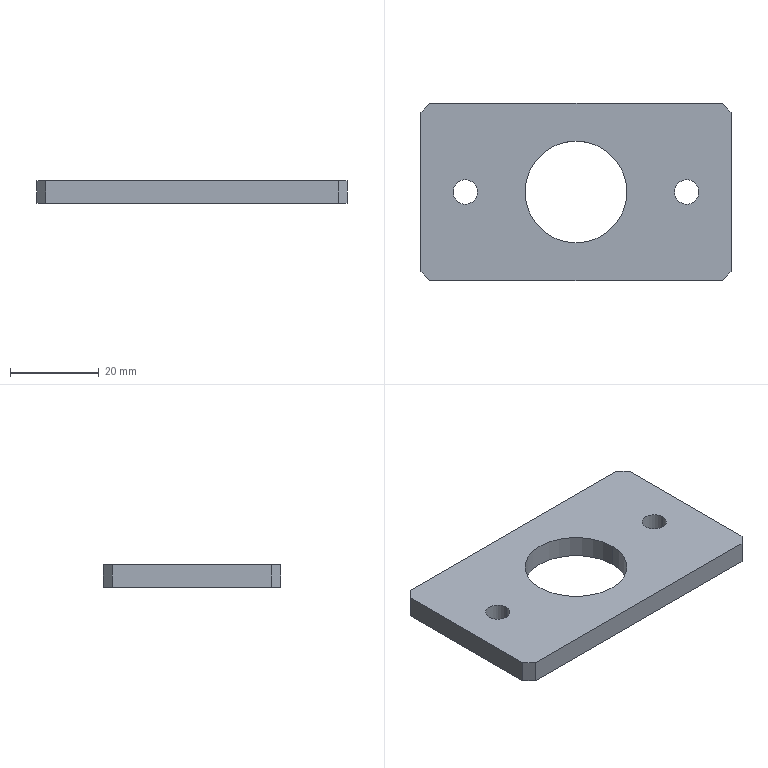Part | SolidWorks | features Chamfer 1, FlatPattern 1, HoleWzd 1, ICE 1, SMBaseFlange 1, SheetMetal 1 | 1 solid | 16 faces | box 70 x 40 x 5 mm | volume 11645 mm3 | plane 10 | cylinder 6 | commonest cylinder face diameters 5.5 x4 23 x2
STEP:
#1=CARTESIAN_POINT('',(22.25,0.,-5.));
#2=VERTEX_POINT('',#1);
#3=CARTESIAN_POINT('',(27.75,0.,-5.));
#4=VERTEX_POINT('',#3);
#5=CARTESIAN_POINT('',(25.,0.,-5.));
#6=DIRECTION('',(0.,0.,1.));
#7=DIRECTION('',(1.,0.,0.));
#8=AXIS2_PLACEMENT_3D('',#5,#6,#7);
#9=CIRCLE('',#8,2.75);
#10=EDGE_CURVE('',#2,#4,#9,.T.);
#11=ORIENTED_EDGE('',*,*,#10,.F.);
#12=CARTESIAN_POINT('',(22.25,0.,0.));
#13=VERTEX_POINT('',#12);
#14=CARTESIAN_POINT('',(22.25,0.,0.));
#15=DIRECTION('',(0.,0.,1.));
#16=VECTOR('',#15,1000.);
#17=LINE('',#14,#16);
#18=EDGE_CURVE('',#2,#13,#17,.T.);
#19=ORIENTED_EDGE('',*,*,#18,.T.);
#20=CARTESIAN_POINT('',(27.75,0.,0.));
#21=VERTEX_POINT('',#20);
#22=CARTESIAN_POINT('',(25.,0.,0.));
#23=DIRECTION('',(0.,0.,1.));
#24=DIRECTION('',(1.,0.,0.));
#25=AXIS2_PLACEMENT_3D('',#22,#23,#24);
#26=CIRCLE('',#25,2.75);
#27=EDGE_CURVE('',#13,#21,#26,.T.);
#28=ORIENTED_EDGE('',*,*,#27,.T.);
#29=CARTESIAN_POINT('',(27.75,0.,0.));
#30=DIRECTION('',(0.,0.,1.));
#31=VECTOR('',#30,1000.);
#32=LINE('',#29,#31);
#33=EDGE_CURVE('',#4,#21,#32,.T.);
#34=ORIENTED_EDGE('',*,*,#33,.F.);
#35=EDGE_LOOP('',(#11,#19,#28,#34));
#36=FACE_OUTER_BOUND('',#35,.T.);
#37=CARTESIAN_POINT('',(25.,0.,0.));
#38=DIRECTION('',(0.,0.,1.));
#39=DIRECTION('',(1.,0.,0.));
#40=AXIS2_PLACEMENT_3D('',#37,#38,#39);
#41=CYLINDRICAL_SURFACE('',#40,2.75);
#42=ADVANCED_FACE('',(#36),#41,.F.);
#43=CARTESIAN_POINT('',(-27.75,0.,-5.));
#44=VERTEX_POINT('',#43);
#45=CARTESIAN_POINT('',(-22.25,0.,-5.));
#46=VERTEX_POINT('',#45);
#47=CARTESIAN_POINT('',(-25.,0.,-5.));
#48=DIRECTION('',(0.,0.,1.));
#49=DIRECTION('',(1.,0.,0.));
#50=AXIS2_PLACEMENT_3D('',#47,#48,#49);
#51=CIRCLE('',#50,2.75);
#52=EDGE_CURVE('',#44,#46,#51,.T.);
#53=ORIENTED_EDGE('',*,*,#52,.F.);
#54=CARTESIAN_POINT('',(-27.75,0.,0.));
#55=VERTEX_POINT('',#54);
#56=CARTESIAN_POINT('',(-27.75,0.,0.));
#57=DIRECTION('',(0.,0.,1.));
#58=VECTOR('',#57,1000.);
#59=LINE('',#56,#58);
#60=EDGE_CURVE('',#44,#55,#59,.T.);
#61=ORIENTED_EDGE('',*,*,#60,.T.);
#62=CARTESIAN_POINT('',(-22.25,0.,0.));
#63=VERTEX_POINT('',#62);
#64=CARTESIAN_POINT('',(-25.,0.,0.));
#65=DIRECTION('',(0.,0.,1.));
#66=DIRECTION('',(1.,0.,0.));
#67=AXIS2_PLACEMENT_3D('',#64,#65,#66);
#68=CIRCLE('',#67,2.75);
#69=EDGE_CURVE('',#55,#63,#68,.T.);
#70=ORIENTED_EDGE('',*,*,#69,.T.);
#71=CARTESIAN_POINT('',(-22.25,0.,0.));
#72=DIRECTION('',(0.,0.,1.));
#73=VECTOR('',#72,1000.);
#74=LINE('',#71,#73);
#75=EDGE_CURVE('',#46,#63,#74,.T.);
#76=ORIENTED_EDGE('',*,*,#75,.F.);
#77=EDGE_LOOP('',(#53,#61,#70,#76));
#78=FACE_OUTER_BOUND('',#77,.T.);
#79=CARTESIAN_POINT('',(-25.,0.,0.));
#80=DIRECTION('',(0.,0.,1.));
#81=DIRECTION('',(1.,0.,0.));
#82=AXIS2_PLACEMENT_3D('',#79,#80,#81);
#83=CYLINDRICAL_SURFACE('',#82,2.75);
#84=ADVANCED_FACE('',(#78),#83,.F.);
#85=CARTESIAN_POINT('',(-11.5,0.,-5.));
#86=VERTEX_POINT('',#85);
#87=CARTESIAN_POINT('',(11.5,0.,-5.));
#88=VERTEX_POINT('',#87);
#89=CARTESIAN_POINT('',(0.,0.,-5.));
#90=DIRECTION('',(0.,0.,1.));
#91=DIRECTION('',(1.,0.,0.));
#92=AXIS2_PLACEMENT_3D('',#89,#90,#91);
#93=CIRCLE('',#92,11.5);
#94=EDGE_CURVE('',#86,#88,#93,.T.);
#95=ORIENTED_EDGE('',*,*,#94,.F.);
#96=CARTESIAN_POINT('',(-11.5,0.,0.));
#97=VERTEX_POINT('',#96);
#98=CARTESIAN_POINT('',(-11.5,0.,-10.));
#99=DIRECTION('',(0.,0.,1.));
#100=VECTOR('',#99,1000.);
#101=LINE('',#98,#100);
#102=EDGE_CURVE('',#86,#97,#101,.T.);
#103=ORIENTED_EDGE('',*,*,#102,.T.);
#104=CARTESIAN_POINT('',(11.5,0.,0.));
#105=VERTEX_POINT('',#104);
#106=CARTESIAN_POINT('',(0.,0.,0.));
#107=DIRECTION('',(0.,0.,1.));
#108=DIRECTION('',(1.,0.,0.));
#109=AXIS2_PLACEMENT_3D('',#106,#107,#108);
#110=CIRCLE('',#109,11.5);
#111=EDGE_CURVE('',#97,#105,#110,.T.);
#112=ORIENTED_EDGE('',*,*,#111,.T.);
#113=CARTESIAN_POINT('',(11.5,0.,-10.));
#114=DIRECTION('',(0.,0.,1.));
#115=VECTOR('',#114,1000.);
#116=LINE('',#113,#115);
#117=EDGE_CURVE('',#88,#105,#116,.T.);
#118=ORIENTED_EDGE('',*,*,#117,.F.);
#119=EDGE_LOOP('',(#95,#103,#112,#118));
#120=FACE_OUTER_BOUND('',#119,.T.);
#121=CARTESIAN_POINT('',(0.,0.,-10.));
#122=DIRECTION('',(0.,0.,1.));
#123=DIRECTION('',(1.,0.,0.));
#124=AXIS2_PLACEMENT_3D('',#121,#122,#123);
#125=CYLINDRICAL_SURFACE('',#124,11.5);
#126=ADVANCED_FACE('',(#120),#125,.F.);
#127=CARTESIAN_POINT('',(35.,-18.,-5.));
#128=VERTEX_POINT('',#127);
#129=CARTESIAN_POINT('',(35.,18.,-5.));
#130=VERTEX_POINT('',#129);
#131=CARTESIAN_POINT('',(35.,20.,-5.));
#132=DIRECTION('',(0.,1.,0.));
#133=VECTOR('',#132,1000.);
#134=LINE('',#131,#133);
#135=EDGE_CURVE('',#128,#130,#134,.T.);
#136=ORIENTED_EDGE('',*,*,#135,.T.);
#137=CARTESIAN_POINT('',(35.,18.,0.));
#138=VERTEX_POINT('',#137);
#139=CARTESIAN_POINT('',(35.,18.,-5.));
#140=DIRECTION('',(0.,0.,1.));
#141=VECTOR('',#140,1000.);
#142=LINE('',#139,#141);
#143=EDGE_CURVE('',#130,#138,#142,.T.);
#144=ORIENTED_EDGE('',*,*,#143,.T.);
#145=CARTESIAN_POINT('',(35.,-18.,0.));
#146=VERTEX_POINT('',#145);
#147=CARTESIAN_POINT('',(35.,20.,0.));
#148=DIRECTION('',(0.,1.,0.));
#149=VECTOR('',#148,1000.);
#150=LINE('',#147,#149);
#151=EDGE_CURVE('',#146,#138,#150,.T.);
#152=ORIENTED_EDGE('',*,*,#151,.F.);
#153=CARTESIAN_POINT('',(35.,-18.,-5.));
#154=DIRECTION('',(0.,0.,-1.));
#155=VECTOR('',#154,1000.);
#156=LINE('',#153,#155);
#157=EDGE_CURVE('',#146,#128,#156,.T.);
#158=ORIENTED_EDGE('',*,*,#157,.T.);
#159=EDGE_LOOP('',(#136,#144,#152,#158));
#160=FACE_OUTER_BOUND('',#159,.T.);
#161=CARTESIAN_POINT('',(35.,20.,-5.));
#162=DIRECTION('',(1.,0.,0.));
#163=DIRECTION('',(0.,1.,0.));
#164=AXIS2_PLACEMENT_3D('',#161,#162,#163);
#165=PLANE('',#164);
#166=ADVANCED_FACE('',(#160),#165,.T.);
#167=CARTESIAN_POINT('',(-33.,-20.,0.));
#168=VERTEX_POINT('',#167);
#169=CARTESIAN_POINT('',(33.,-20.,0.));
#170=VERTEX_POINT('',#169);
#171=CARTESIAN_POINT('',(-35.,-20.,0.));
#172=DIRECTION('',(1.,0.,0.));
#173=VECTOR('',#172,1000.);
#174=LINE('',#171,#173);
#175=EDGE_CURVE('',#168,#170,#174,.T.);
#176=ORIENTED_EDGE('',*,*,#175,.F.);
#177=CARTESIAN_POINT('',(-33.,-20.,-5.));
#178=VERTEX_POINT('',#177);
#179=CARTESIAN_POINT('',(-33.,-20.,-5.));
#180=DIRECTION('',(0.,0.,-1.));
#181=VECTOR('',#180,1000.);
#182=LINE('',#179,#181);
#183=EDGE_CURVE('',#168,#178,#182,.T.);
#184=ORIENTED_EDGE('',*,*,#183,.T.);
#185=CARTESIAN_POINT('',(33.,-20.,-5.));
#186=VERTEX_POINT('',#185);
#187=CARTESIAN_POINT('',(-35.,-20.,-5.));
#188=DIRECTION('',(1.,0.,0.));
#189=VECTOR('',#188,1000.);
#190=LINE('',#187,#189);
#191=EDGE_CURVE('',#178,#186,#190,.T.);
#192=ORIENTED_EDGE('',*,*,#191,.T.);
#193=CARTESIAN_POINT('',(33.,-20.,-5.));
#194=DIRECTION('',(0.,0.,1.));
#195=VECTOR('',#194,1000.);
#196=LINE('',#193,#195);
#197=EDGE_CURVE('',#186,#170,#196,.T.);
#198=ORIENTED_EDGE('',*,*,#197,.T.);
#199=EDGE_LOOP('',(#176,#184,#192,#198));
#200=FACE_OUTER_BOUND('',#199,.T.);
#201=CARTESIAN_POINT('',(-35.,-20.,-5.));
#202=DIRECTION('',(0.,-1.,0.));
#203=DIRECTION('',(0.,0.,-1.));
#204=AXIS2_PLACEMENT_3D('',#201,#202,#203);
#205=PLANE('',#204);
#206=ADVANCED_FACE('',(#200),#205,.T.);
#207=CARTESIAN_POINT('',(-35.,18.,0.));
#208=VERTEX_POINT('',#207);
#209=CARTESIAN_POINT('',(-35.,-18.,0.));
#210=VERTEX_POINT('',#209);
#211=CARTESIAN_POINT('',(-35.,20.,0.));
#212=DIRECTION('',(0.,-1.,0.));
#213=VECTOR('',#212,1000.);
#214=LINE('',#211,#213);
#215=EDGE_CURVE('',#208,#210,#214,.T.);
#216=ORIENTED_EDGE('',*,*,#215,.F.);
#217=CARTESIAN_POINT('',(-35.,18.,-5.));
#218=VERTEX_POINT('',#217);
#219=CARTESIAN_POINT('',(-35.,18.,-5.));
#220=DIRECTION('',(0.,0.,-1.));
#221=VECTOR('',#220,1000.);
#222=LINE('',#219,#221);
#223=EDGE_CURVE('',#208,#218,#222,.T.);
#224=ORIENTED_EDGE('',*,*,#223,.T.);
#225=CARTESIAN_POINT('',(-35.,-18.,-5.));
#226=VERTEX_POINT('',#225);
#227=CARTESIAN_POINT('',(-35.,20.,-5.));
#228=DIRECTION('',(0.,-1.,0.));
#229=VECTOR('',#228,1000.);
#230=LINE('',#227,#229);
#231=EDGE_CURVE('',#218,#226,#230,.T.);
#232=ORIENTED_EDGE('',*,*,#231,.T.);
#233=CARTESIAN_POINT('',(-35.,-18.,-5.));
#234=DIRECTION('',(0.,0.,1.));
#235=VECTOR('',#234,1000.);
#236=LINE('',#233,#235);
#237=EDGE_CURVE('',#226,#210,#236,.T.);
#238=ORIENTED_EDGE('',*,*,#237,.T.);
#239=EDGE_LOOP('',(#216,#224,#232,#238));
#240=FACE_OUTER_BOUND('',#239,.T.);
#241=CARTESIAN_POINT('',(-35.,20.,-5.));
#242=DIRECTION('',(-1.,0.,0.));
#243=DIRECTION('',(0.,-1.,0.));
#244=AXIS2_PLACEMENT_3D('',#241,#242,#243);
#245=PLANE('',#244);
#246=ADVANCED_FACE('',(#240),#245,.T.);
#247=CARTESIAN_POINT('',(33.,20.,0.));
#248=VERTEX_POINT('',#247);
#249=CARTESIAN_POINT('',(-33.,20.,0.));
#250=VERTEX_POINT('',#249);
#251=CARTESIAN_POINT('',(-35.,20.,0.));
#252=DIRECTION('',(-1.,0.,0.));
#253=VECTOR('',#252,1000.);
#254=LINE('',#251,#253);
#255=EDGE_CURVE('',#248,#250,#254,.T.);
#256=ORIENTED_EDGE('',*,*,#255,.F.);
#257=CARTESIAN_POINT('',(33.,20.,-5.));
#258=VERTEX_POINT('',#257);
#259=CARTESIAN_POINT('',(33.,20.,-5.));
#260=DIRECTION('',(0.,0.,-1.));
#261=VECTOR('',#260,1000.);
#262=LINE('',#259,#261);
#263=EDGE_CURVE('',#248,#258,#262,.T.);
#264=ORIENTED_EDGE('',*,*,#263,.T.);
#265=CARTESIAN_POINT('',(-33.,20.,-5.));
#266=VERTEX_POINT('',#265);
#267=CARTESIAN_POINT('',(-35.,20.,-5.));
#268=DIRECTION('',(-1.,0.,0.));
#269=VECTOR('',#268,1000.);
#270=LINE('',#267,#269);
#271=EDGE_CURVE('',#258,#266,#270,.T.);
#272=ORIENTED_EDGE('',*,*,#271,.T.);
#273=CARTESIAN_POINT('',(-33.,20.,-5.));
#274=DIRECTION('',(0.,0.,1.));
#275=VECTOR('',#274,1000.);
#276=LINE('',#273,#275);
#277=EDGE_CURVE('',#266,#250,#276,.T.);
#278=ORIENTED_EDGE('',*,*,#277,.T.);
#279=EDGE_LOOP('',(#256,#264,#272,#278));
#280=FACE_OUTER_BOUND('',#279,.T.);
#281=CARTESIAN_POINT('',(-35.,20.,-5.));
#282=DIRECTION('',(0.,1.,0.));
#283=DIRECTION('',(0.,0.,1.));
#284=AXIS2_PLACEMENT_3D('',#281,#282,#283);
#285=PLANE('',#284);
#286=ADVANCED_FACE('',(#280),#285,.T.);
#287=CARTESIAN_POINT('',(25.,0.,-5.));
#288=DIRECTION('',(0.,0.,1.));
#289=DIRECTION('',(1.,0.,0.));
#290=AXIS2_PLACEMENT_3D('',#287,#288,#289);
#291=CIRCLE('',#290,2.75);
#292=EDGE_CURVE('',#4,#2,#291,.T.);
#293=ORIENTED_EDGE('',*,*,#292,.T.);
#294=ORIENTED_EDGE('',*,*,#10,.T.);
#295=EDGE_LOOP('',(#293,#294));
#296=FACE_BOUND('',#295,.T.);
#297=CARTESIAN_POINT('',(-25.,0.,-5.));
#298=DIRECTION('',(0.,0.,1.));
#299=DIRECTION('',(1.,0.,0.));
#300=AXIS2_PLACEMENT_3D('',#297,#298,#299);
#301=CIRCLE('',#300,2.75);
#302=EDGE_CURVE('',#46,#44,#301,.T.);
#303=ORIENTED_EDGE('',*,*,#302,.T.);
#304=ORIENTED_EDGE('',*,*,#52,.T.);
#305=EDGE_LOOP('',(#303,#304));
#306=FACE_BOUND('',#305,.T.);
#307=CARTESIAN_POINT('',(0.,0.,-5.));
#308=DIRECTION('',(0.,0.,1.));
#309=DIRECTION('',(1.,0.,0.));
#310=AXIS2_PLACEMENT_3D('',#307,#308,#309);
#311=CIRCLE('',#310,11.5);
#312=EDGE_CURVE('',#88,#86,#311,.T.);
#313=ORIENTED_EDGE('',*,*,#312,.T.);
#314=ORIENTED_EDGE('',*,*,#94,.T.);
#315=EDGE_LOOP('',(#313,#314));
#316=FACE_BOUND('',#315,.T.);
#317=ORIENTED_EDGE('',*,*,#271,.F.);
#318=CARTESIAN_POINT('',(35.,18.,-5.));
#319=DIRECTION('',(0.7071,-0.7071,0.));
#320=VECTOR('',#319,1000.);
#321=LINE('',#318,#320);
#322=EDGE_CURVE('',#258,#130,#321,.T.);
#323=ORIENTED_EDGE('',*,*,#322,.T.);
#324=ORIENTED_EDGE('',*,*,#135,.F.);
#325=CARTESIAN_POINT('',(33.,-20.,-5.));
#326=DIRECTION('',(-0.7071,-0.7071,0.));
#327=VECTOR('',#326,1000.);
#328=LINE('',#325,#327);
#329=EDGE_CURVE('',#128,#186,#328,.T.);
#330=ORIENTED_EDGE('',*,*,#329,.T.);
#331=ORIENTED_EDGE('',*,*,#191,.F.);
#332=CARTESIAN_POINT('',(-35.,-18.,-5.));
#333=DIRECTION('',(-0.7071,0.7071,0.));
#334=VECTOR('',#333,1000.);
#335=LINE('',#332,#334);
#336=EDGE_CURVE('',#178,#226,#335,.T.);
#337=ORIENTED_EDGE('',*,*,#336,.T.);
#338=ORIENTED_EDGE('',*,*,#231,.F.);
#339=CARTESIAN_POINT('',(-33.,20.,-5.));
#340=DIRECTION('',(0.7071,0.7071,0.));
#341=VECTOR('',#340,1000.);
#342=LINE('',#339,#341);
#343=EDGE_CURVE('',#218,#266,#342,.T.);
#344=ORIENTED_EDGE('',*,*,#343,.T.);
#345=EDGE_LOOP('',(#317,#323,#324,#330,#331,#337,#338,#344));
#346=FACE_OUTER_BOUND('',#345,.T.);
#347=CARTESIAN_POINT('',(0.,0.,-5.));
#348=DIRECTION('',(0.,0.,1.));
#349=DIRECTION('',(1.,0.,0.));
#350=AXIS2_PLACEMENT_3D('',#347,#348,#349);
#351=PLANE('',#350);
#352=ADVANCED_FACE('',(#296,#306,#316,#346),#351,.F.);
#353=CARTESIAN_POINT('',(25.,0.,0.));
#354=DIRECTION('',(0.,0.,1.));
#355=DIRECTION('',(1.,0.,0.));
#356=AXIS2_PLACEMENT_3D('',#353,#354,#355);
#357=CIRCLE('',#356,2.75);
#358=EDGE_CURVE('',#21,#13,#357,.T.);
#359=ORIENTED_EDGE('',*,*,#358,.F.);
#360=ORIENTED_EDGE('',*,*,#27,.F.);
#361=EDGE_LOOP('',(#359,#360));
#362=FACE_BOUND('',#361,.T.);
#363=CARTESIAN_POINT('',(-25.,0.,0.));
#364=DIRECTION('',(0.,0.,1.));
#365=DIRECTION('',(1.,0.,0.));
#366=AXIS2_PLACEMENT_3D('',#363,#364,#365);
#367=CIRCLE('',#366,2.75);
#368=EDGE_CURVE('',#63,#55,#367,.T.);
#369=ORIENTED_EDGE('',*,*,#368,.F.);
#370=ORIENTED_EDGE('',*,*,#69,.F.);
#371=EDGE_LOOP('',(#369,#370));
#372=FACE_BOUND('',#371,.T.);
#373=CARTESIAN_POINT('',(0.,0.,0.));
#374=DIRECTION('',(0.,0.,1.));
#375=DIRECTION('',(1.,0.,0.));
#376=AXIS2_PLACEMENT_3D('',#373,#374,#375);
#377=CIRCLE('',#376,11.5);
#378=EDGE_CURVE('',#105,#97,#377,.T.);
#379=ORIENTED_EDGE('',*,*,#378,.F.);
#380=ORIENTED_EDGE('',*,*,#111,.F.);
#381=EDGE_LOOP('',(#379,#380));
#382=FACE_BOUND('',#381,.T.);
#383=ORIENTED_EDGE('',*,*,#151,.T.);
#384=CARTESIAN_POINT('',(26.5,26.5,0.));
#385=DIRECTION('',(-0.7071,0.7071,0.));
#386=VECTOR('',#385,1000.);
#387=LINE('',#384,#386);
#388=EDGE_CURVE('',#138,#248,#387,.T.);
#389=ORIENTED_EDGE('',*,*,#388,.T.);
#390=ORIENTED_EDGE('',*,*,#255,.T.);
#391=CARTESIAN_POINT('',(-26.5,26.5,0.));
#392=DIRECTION('',(-0.7071,-0.7071,0.));
#393=VECTOR('',#392,1000.);
#394=LINE('',#391,#393);
#395=EDGE_CURVE('',#250,#208,#394,.T.);
#396=ORIENTED_EDGE('',*,*,#395,.T.);
#397=ORIENTED_EDGE('',*,*,#215,.T.);
#398=CARTESIAN_POINT('',(-26.5,-26.5,0.));
#399=DIRECTION('',(0.7071,-0.7071,0.));
#400=VECTOR('',#399,1000.);
#401=LINE('',#398,#400);
#402=EDGE_CURVE('',#210,#168,#401,.T.);
#403=ORIENTED_EDGE('',*,*,#402,.T.);
#404=ORIENTED_EDGE('',*,*,#175,.T.);
#405=CARTESIAN_POINT('',(26.5,-26.5,0.));
#406=DIRECTION('',(0.7071,0.7071,0.));
#407=VECTOR('',#406,1000.);
#408=LINE('',#405,#407);
#409=EDGE_CURVE('',#170,#146,#408,.T.);
#410=ORIENTED_EDGE('',*,*,#409,.T.);
#411=EDGE_LOOP('',(#383,#389,#390,#396,#397,#403,#404,#410));
#412=FACE_OUTER_BOUND('',#411,.T.);
#413=CARTESIAN_POINT('',(0.,0.,0.));
#414=DIRECTION('',(0.,0.,1.));
#415=DIRECTION('',(1.,0.,0.));
#416=AXIS2_PLACEMENT_3D('',#413,#414,#415);
#417=PLANE('',#416);
#418=ADVANCED_FACE('',(#362,#372,#382,#412),#417,.T.);
#419=ORIENTED_EDGE('',*,*,#102,.F.);
#420=ORIENTED_EDGE('',*,*,#312,.F.);
#421=ORIENTED_EDGE('',*,*,#117,.T.);
#422=ORIENTED_EDGE('',*,*,#378,.T.);
#423=EDGE_LOOP('',(#419,#420,#421,#422));
#424=FACE_OUTER_BOUND('',#423,.T.);
#425=CARTESIAN_POINT('',(0.,0.,-10.));
#426=DIRECTION('',(0.,0.,1.));
#427=DIRECTION('',(1.,0.,0.));
#428=AXIS2_PLACEMENT_3D('',#425,#426,#427);
#429=CYLINDRICAL_SURFACE('',#428,11.5);
#430=ADVANCED_FACE('',(#424),#429,.F.);
#431=ORIENTED_EDGE('',*,*,#60,.F.);
#432=ORIENTED_EDGE('',*,*,#302,.F.);
#433=ORIENTED_EDGE('',*,*,#75,.T.);
#434=ORIENTED_EDGE('',*,*,#368,.T.);
#435=EDGE_LOOP('',(#431,#432,#433,#434));
#436=FACE_OUTER_BOUND('',#435,.T.);
#437=CARTESIAN_POINT('',(-25.,0.,0.));
#438=DIRECTION('',(0.,0.,1.));
#439=DIRECTION('',(1.,0.,0.));
#440=AXIS2_PLACEMENT_3D('',#437,#438,#439);
#441=CYLINDRICAL_SURFACE('',#440,2.75);
#442=ADVANCED_FACE('',(#436),#441,.F.);
#443=ORIENTED_EDGE('',*,*,#18,.F.);
#444=ORIENTED_EDGE('',*,*,#292,.F.);
#445=ORIENTED_EDGE('',*,*,#33,.T.);
#446=ORIENTED_EDGE('',*,*,#358,.T.);
#447=EDGE_LOOP('',(#443,#444,#445,#446));
#448=FACE_OUTER_BOUND('',#447,.T.);
#449=CARTESIAN_POINT('',(25.,0.,0.));
#450=DIRECTION('',(0.,0.,1.));
#451=DIRECTION('',(1.,0.,0.));
#452=AXIS2_PLACEMENT_3D('',#449,#450,#451);
#453=CYLINDRICAL_SURFACE('',#452,2.75);
#454=ADVANCED_FACE('',(#448),#453,.F.);
#455=ORIENTED_EDGE('',*,*,#322,.F.);
#456=ORIENTED_EDGE('',*,*,#263,.F.);
#457=ORIENTED_EDGE('',*,*,#388,.F.);
#458=ORIENTED_EDGE('',*,*,#143,.F.);
#459=EDGE_LOOP('',(#455,#456,#457,#458));
#460=FACE_OUTER_BOUND('',#459,.T.);
#461=CARTESIAN_POINT('',(35.,18.,-5.));
#462=DIRECTION('',(-0.7071,-0.7071,0.));
#463=DIRECTION('',(0.,0.,1.));
#464=AXIS2_PLACEMENT_3D('',#461,#462,#463);
#465=PLANE('',#464);
#466=ADVANCED_FACE('',(#460),#465,.F.);
#467=ORIENTED_EDGE('',*,*,#343,.F.);
#468=ORIENTED_EDGE('',*,*,#223,.F.);
#469=ORIENTED_EDGE('',*,*,#395,.F.);
#470=ORIENTED_EDGE('',*,*,#277,.F.);
#471=EDGE_LOOP('',(#467,#468,#469,#470));
#472=FACE_OUTER_BOUND('',#471,.T.);
#473=CARTESIAN_POINT('',(-33.,20.,-5.));
#474=DIRECTION('',(0.7071,-0.7071,0.));
#475=DIRECTION('',(0.,0.,1.));
#476=AXIS2_PLACEMENT_3D('',#473,#474,#475);
#477=PLANE('',#476);
#478=ADVANCED_FACE('',(#472),#477,.F.);
#479=ORIENTED_EDGE('',*,*,#336,.F.);
#480=ORIENTED_EDGE('',*,*,#183,.F.);
#481=ORIENTED_EDGE('',*,*,#402,.F.);
#482=ORIENTED_EDGE('',*,*,#237,.F.);
#483=EDGE_LOOP('',(#479,#480,#481,#482));
#484=FACE_OUTER_BOUND('',#483,.T.);
#485=CARTESIAN_POINT('',(-35.,-18.,-5.));
#486=DIRECTION('',(0.7071,0.7071,0.));
#487=DIRECTION('',(0.,0.,1.));
#488=AXIS2_PLACEMENT_3D('',#485,#486,#487);
#489=PLANE('',#488);
#490=ADVANCED_FACE('',(#484),#489,.F.);
#491=ORIENTED_EDGE('',*,*,#329,.F.);
#492=ORIENTED_EDGE('',*,*,#157,.F.);
#493=ORIENTED_EDGE('',*,*,#409,.F.);
#494=ORIENTED_EDGE('',*,*,#197,.F.);
#495=EDGE_LOOP('',(#491,#492,#493,#494));
#496=FACE_OUTER_BOUND('',#495,.T.);
#497=CARTESIAN_POINT('',(33.,-20.,-5.));
#498=DIRECTION('',(-0.7071,0.7071,0.));
#499=DIRECTION('',(0.,0.,1.));
#500=AXIS2_PLACEMENT_3D('',#497,#498,#499);
#501=PLANE('',#500);
#502=ADVANCED_FACE('',(#496),#501,.F.);
#503=CLOSED_SHELL('',(#42,#84,#126,#166,#206,#246,#286,#352,#418,#430,#442,#454,#466,#478,#490,#502));
#504=MANIFOLD_SOLID_BREP('',#503);
#505=CARTESIAN_POINT('',(0.,0.,0.));
#506=DIRECTION('',(0.,0.,1.));
#507=DIRECTION('',(1.,0.,0.));
#508=AXIS2_PLACEMENT_3D('',#505,#506,#507);
#509=(LENGTH_UNIT()NAMED_UNIT(*)SI_UNIT(.MILLI.,.METRE.));
#510=UNCERTAINTY_MEASURE_WITH_UNIT(LENGTH_MEASURE(0.00001),#509,'','');
#511=(NAMED_UNIT(*)PLANE_ANGLE_UNIT()SI_UNIT($,.RADIAN.));
#512=(NAMED_UNIT(*)SI_UNIT($,.STERADIAN.)SOLID_ANGLE_UNIT());
#513=(GEOMETRIC_REPRESENTATION_CONTEXT(3)GLOBAL_UNCERTAINTY_ASSIGNED_CONTEXT((#510))GLOBAL_UNIT_ASSIGNED_CONTEXT((#509,#511,#512))REPRESENTATION_CONTEXT('',''));
#514=ADVANCED_BREP_SHAPE_REPRESENTATION('',(#504,#508),#513);